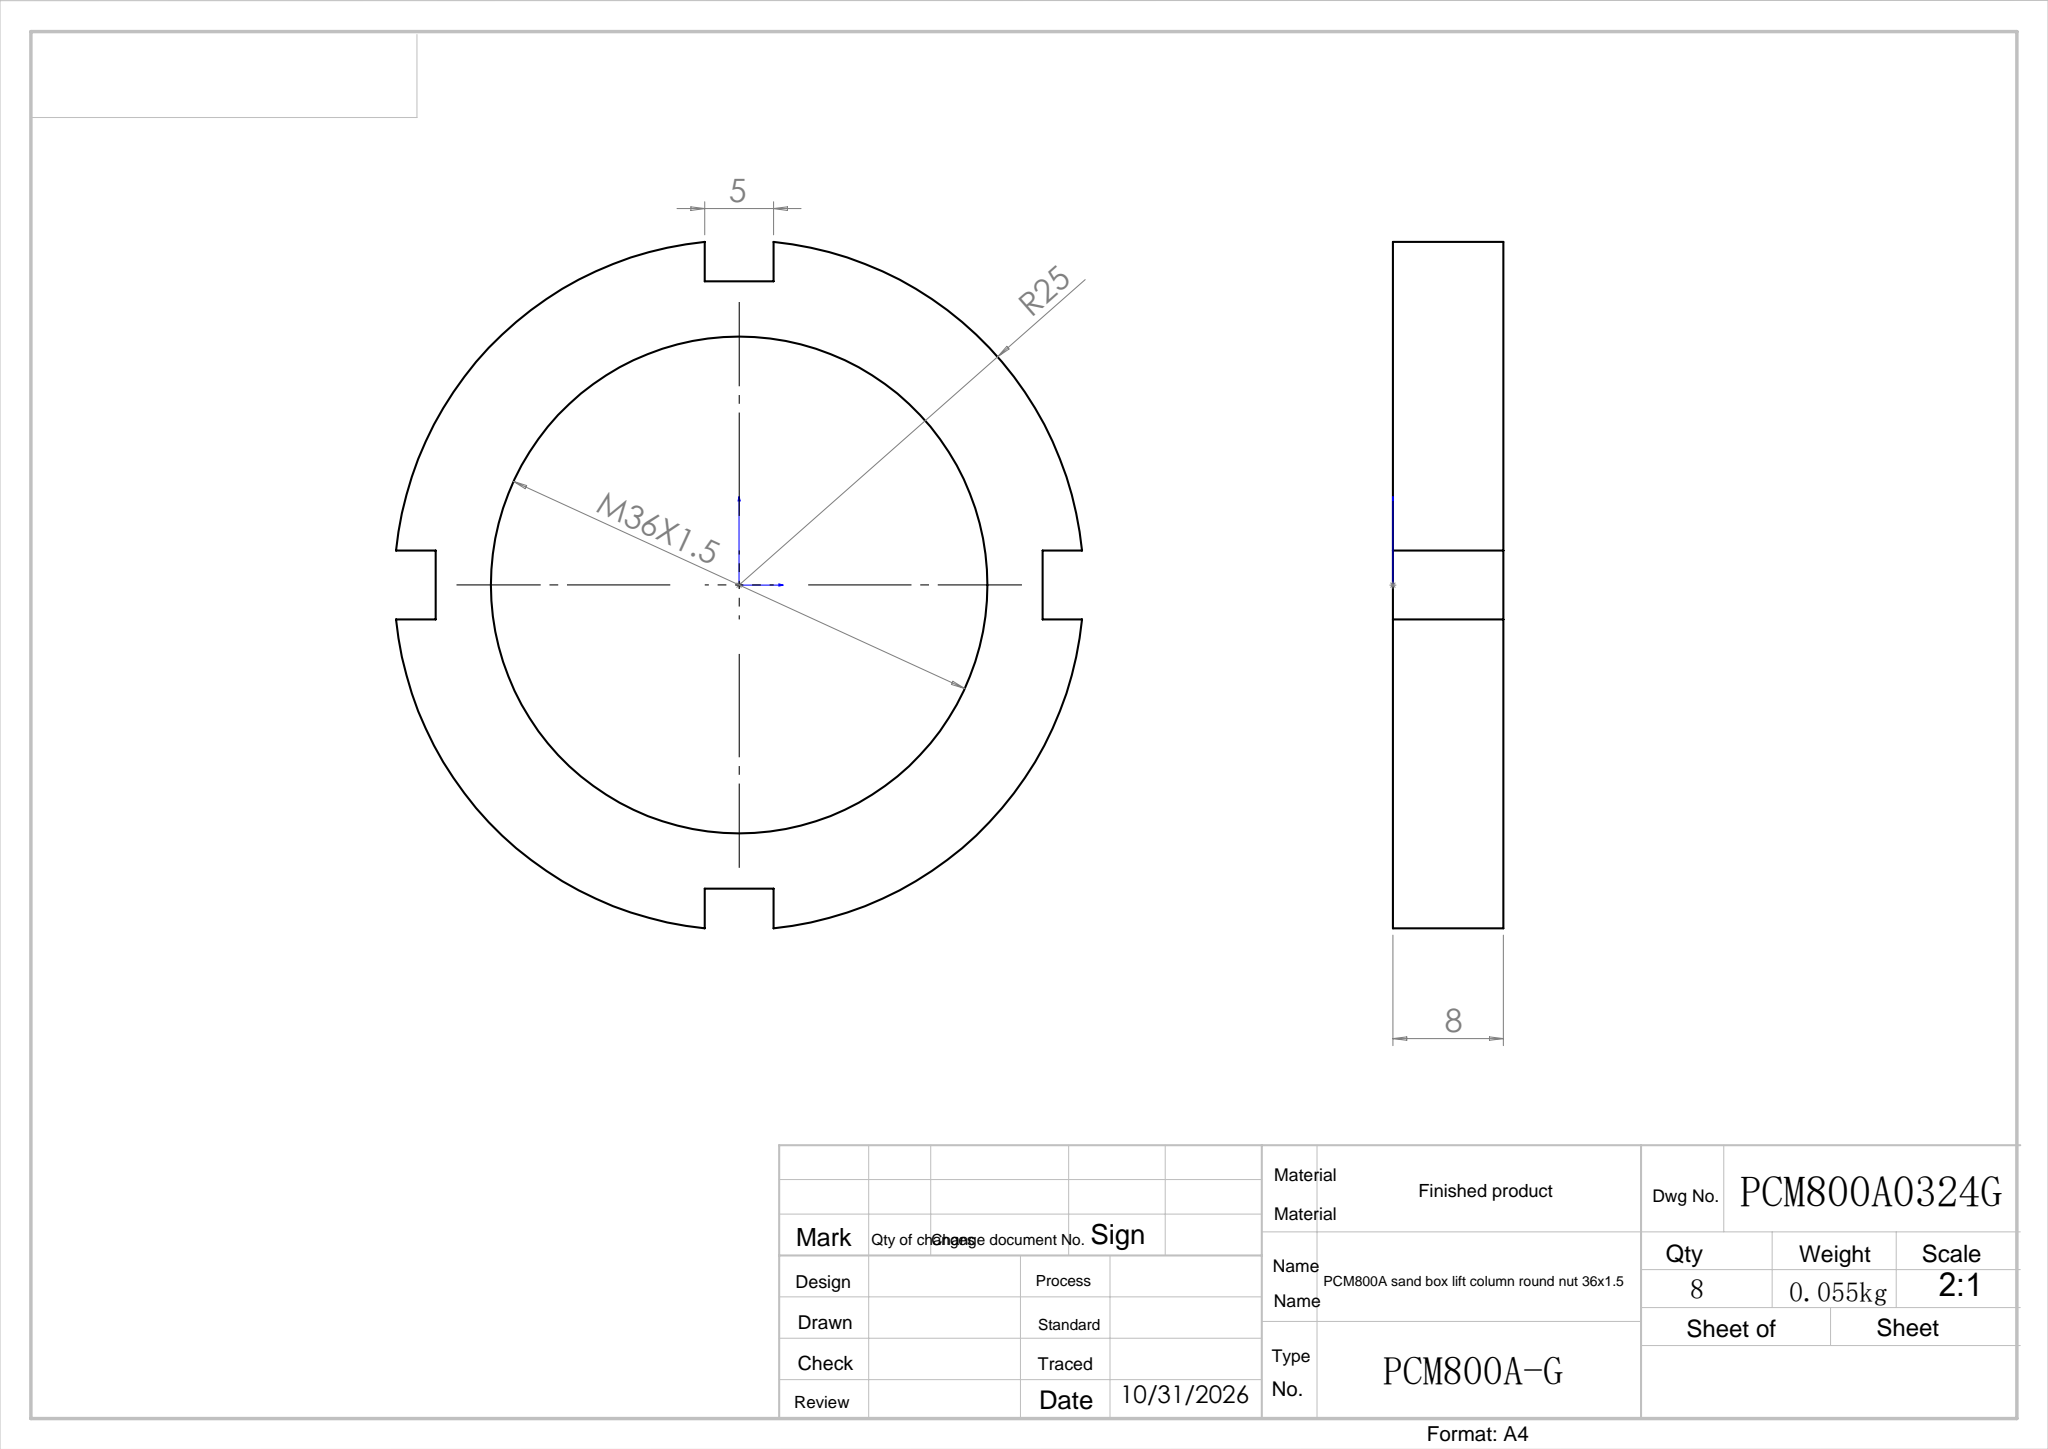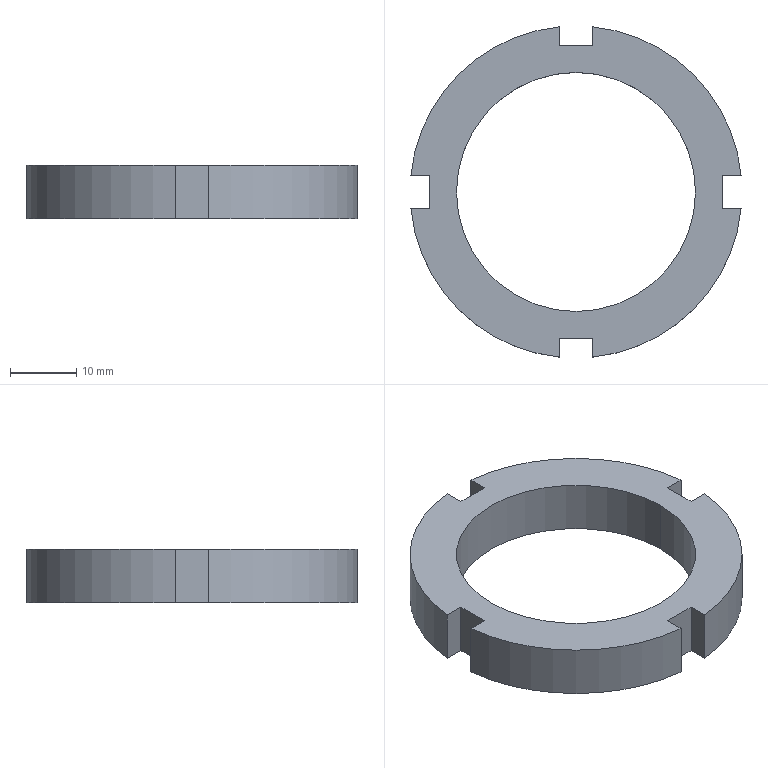Part | SolidWorks | features Extrusion 1 | 1 solid | 20 faces | box 49.742 x 49.742 x 8 mm | volume 7088 mm3 | plane 14 | cylinder 6 | commonest cylinder face diameters 49.993 x4 36 x2
STEP:
#1=CARTESIAN_POINT('',(-18.,0.,8.));
#2=VERTEX_POINT('',#1);
#3=CARTESIAN_POINT('',(18.,0.,8.));
#4=VERTEX_POINT('',#3);
#5=CARTESIAN_POINT('',(0.,0.,8.));
#6=DIRECTION('',(0.,0.,1.));
#7=DIRECTION('',(1.,0.,0.));
#8=AXIS2_PLACEMENT_3D('',#5,#6,#7);
#9=CIRCLE('',#8,18.);
#10=EDGE_CURVE('',#2,#4,#9,.T.);
#11=ORIENTED_EDGE('',*,*,#10,.T.);
#12=CARTESIAN_POINT('',(18.,0.,0.));
#13=VERTEX_POINT('',#12);
#14=CARTESIAN_POINT('',(18.,0.,8.));
#15=DIRECTION('',(0.,0.,-1.));
#16=VECTOR('',#15,1000.);
#17=LINE('',#14,#16);
#18=EDGE_CURVE('',#4,#13,#17,.T.);
#19=ORIENTED_EDGE('',*,*,#18,.T.);
#20=CARTESIAN_POINT('',(-18.,0.,0.));
#21=VERTEX_POINT('',#20);
#22=CARTESIAN_POINT('',(0.,0.,0.));
#23=DIRECTION('',(0.,0.,1.));
#24=DIRECTION('',(1.,0.,0.));
#25=AXIS2_PLACEMENT_3D('',#22,#23,#24);
#26=CIRCLE('',#25,18.);
#27=EDGE_CURVE('',#21,#13,#26,.T.);
#28=ORIENTED_EDGE('',*,*,#27,.F.);
#29=CARTESIAN_POINT('',(-18.,0.,8.));
#30=DIRECTION('',(0.,0.,-1.));
#31=VECTOR('',#30,1000.);
#32=LINE('',#29,#31);
#33=EDGE_CURVE('',#2,#21,#32,.T.);
#34=ORIENTED_EDGE('',*,*,#33,.F.);
#35=EDGE_LOOP('',(#11,#19,#28,#34));
#36=FACE_OUTER_BOUND('',#35,.T.);
#37=CARTESIAN_POINT('',(0.,0.,8.));
#38=DIRECTION('',(0.,0.,-1.));
#39=DIRECTION('',(-1.,0.,0.));
#40=AXIS2_PLACEMENT_3D('',#37,#38,#39);
#41=CYLINDRICAL_SURFACE('',#40,18.);
#42=ADVANCED_FACE('',(#36),#41,.F.);
#43=CARTESIAN_POINT('',(-2.5,24.871,8.));
#44=VERTEX_POINT('',#43);
#45=CARTESIAN_POINT('',(-24.871,2.5,8.));
#46=VERTEX_POINT('',#45);
#47=CARTESIAN_POINT('',(0.,0.,8.));
#48=DIRECTION('',(0.,0.,1.));
#49=DIRECTION('',(1.,0.,0.));
#50=AXIS2_PLACEMENT_3D('',#47,#48,#49);
#51=CIRCLE('',#50,24.996);
#52=EDGE_CURVE('',#44,#46,#51,.T.);
#53=ORIENTED_EDGE('',*,*,#52,.T.);
#54=CARTESIAN_POINT('',(-22.,2.5,8.));
#55=VERTEX_POINT('',#54);
#56=CARTESIAN_POINT('',(-22.,2.5,8.));
#57=DIRECTION('',(1.,0.,0.));
#58=VECTOR('',#57,1000.);
#59=LINE('',#56,#58);
#60=EDGE_CURVE('',#46,#55,#59,.T.);
#61=ORIENTED_EDGE('',*,*,#60,.T.);
#62=CARTESIAN_POINT('',(-22.,-2.5,8.));
#63=VERTEX_POINT('',#62);
#64=CARTESIAN_POINT('',(-22.,-2.5,8.));
#65=DIRECTION('',(0.,-1.,0.));
#66=VECTOR('',#65,1000.);
#67=LINE('',#64,#66);
#68=EDGE_CURVE('',#55,#63,#67,.T.);
#69=ORIENTED_EDGE('',*,*,#68,.T.);
#70=CARTESIAN_POINT('',(-24.871,-2.5,8.));
#71=VERTEX_POINT('',#70);
#72=CARTESIAN_POINT('',(-24.871,-2.5,8.));
#73=DIRECTION('',(-1.,0.,0.));
#74=VECTOR('',#73,1000.);
#75=LINE('',#72,#74);
#76=EDGE_CURVE('',#63,#71,#75,.T.);
#77=ORIENTED_EDGE('',*,*,#76,.T.);
#78=CARTESIAN_POINT('',(-2.5,-24.871,8.));
#79=VERTEX_POINT('',#78);
#80=CARTESIAN_POINT('',(0.,0.,8.));
#81=DIRECTION('',(0.,0.,1.));
#82=DIRECTION('',(1.,0.,0.));
#83=AXIS2_PLACEMENT_3D('',#80,#81,#82);
#84=CIRCLE('',#83,24.996);
#85=EDGE_CURVE('',#71,#79,#84,.T.);
#86=ORIENTED_EDGE('',*,*,#85,.T.);
#87=CARTESIAN_POINT('',(-2.5,-22.,8.));
#88=VERTEX_POINT('',#87);
#89=CARTESIAN_POINT('',(-2.5,-22.,8.));
#90=DIRECTION('',(0.,1.,0.));
#91=VECTOR('',#90,1000.);
#92=LINE('',#89,#91);
#93=EDGE_CURVE('',#79,#88,#92,.T.);
#94=ORIENTED_EDGE('',*,*,#93,.T.);
#95=CARTESIAN_POINT('',(2.5,-22.,8.));
#96=VERTEX_POINT('',#95);
#97=CARTESIAN_POINT('',(2.5,-22.,8.));
#98=DIRECTION('',(1.,0.,0.));
#99=VECTOR('',#98,1000.);
#100=LINE('',#97,#99);
#101=EDGE_CURVE('',#88,#96,#100,.T.);
#102=ORIENTED_EDGE('',*,*,#101,.T.);
#103=CARTESIAN_POINT('',(2.5,-24.871,8.));
#104=VERTEX_POINT('',#103);
#105=CARTESIAN_POINT('',(2.5,-24.871,8.));
#106=DIRECTION('',(0.,-1.,0.));
#107=VECTOR('',#106,1000.);
#108=LINE('',#105,#107);
#109=EDGE_CURVE('',#96,#104,#108,.T.);
#110=ORIENTED_EDGE('',*,*,#109,.T.);
#111=CARTESIAN_POINT('',(24.871,-2.5,8.));
#112=VERTEX_POINT('',#111);
#113=CARTESIAN_POINT('',(0.,0.,8.));
#114=DIRECTION('',(0.,0.,1.));
#115=DIRECTION('',(1.,0.,0.));
#116=AXIS2_PLACEMENT_3D('',#113,#114,#115);
#117=CIRCLE('',#116,24.996);
#118=EDGE_CURVE('',#104,#112,#117,.T.);
#119=ORIENTED_EDGE('',*,*,#118,.T.);
#120=CARTESIAN_POINT('',(22.,-2.5,8.));
#121=VERTEX_POINT('',#120);
#122=CARTESIAN_POINT('',(22.,-2.5,8.));
#123=DIRECTION('',(-1.,0.,0.));
#124=VECTOR('',#123,1000.);
#125=LINE('',#122,#124);
#126=EDGE_CURVE('',#112,#121,#125,.T.);
#127=ORIENTED_EDGE('',*,*,#126,.T.);
#128=CARTESIAN_POINT('',(22.,2.5,8.));
#129=VERTEX_POINT('',#128);
#130=CARTESIAN_POINT('',(22.,2.5,8.));
#131=DIRECTION('',(0.,1.,0.));
#132=VECTOR('',#131,1000.);
#133=LINE('',#130,#132);
#134=EDGE_CURVE('',#121,#129,#133,.T.);
#135=ORIENTED_EDGE('',*,*,#134,.T.);
#136=CARTESIAN_POINT('',(24.871,2.5,8.));
#137=VERTEX_POINT('',#136);
#138=CARTESIAN_POINT('',(24.871,2.5,8.));
#139=DIRECTION('',(1.,0.,0.));
#140=VECTOR('',#139,1000.);
#141=LINE('',#138,#140);
#142=EDGE_CURVE('',#129,#137,#141,.T.);
#143=ORIENTED_EDGE('',*,*,#142,.T.);
#144=CARTESIAN_POINT('',(2.5,24.871,8.));
#145=VERTEX_POINT('',#144);
#146=CARTESIAN_POINT('',(0.,0.,8.));
#147=DIRECTION('',(0.,0.,1.));
#148=DIRECTION('',(1.,0.,0.));
#149=AXIS2_PLACEMENT_3D('',#146,#147,#148);
#150=CIRCLE('',#149,24.996);
#151=EDGE_CURVE('',#137,#145,#150,.T.);
#152=ORIENTED_EDGE('',*,*,#151,.T.);
#153=CARTESIAN_POINT('',(2.5,22.,8.));
#154=VERTEX_POINT('',#153);
#155=CARTESIAN_POINT('',(2.5,22.,8.));
#156=DIRECTION('',(0.,-1.,0.));
#157=VECTOR('',#156,1000.);
#158=LINE('',#155,#157);
#159=EDGE_CURVE('',#145,#154,#158,.T.);
#160=ORIENTED_EDGE('',*,*,#159,.T.);
#161=CARTESIAN_POINT('',(-2.5,22.,8.));
#162=VERTEX_POINT('',#161);
#163=CARTESIAN_POINT('',(-2.5,22.,8.));
#164=DIRECTION('',(-1.,0.,0.));
#165=VECTOR('',#164,1000.);
#166=LINE('',#163,#165);
#167=EDGE_CURVE('',#154,#162,#166,.T.);
#168=ORIENTED_EDGE('',*,*,#167,.T.);
#169=CARTESIAN_POINT('',(-2.5,24.871,8.));
#170=DIRECTION('',(0.,1.,0.));
#171=VECTOR('',#170,1000.);
#172=LINE('',#169,#171);
#173=EDGE_CURVE('',#162,#44,#172,.T.);
#174=ORIENTED_EDGE('',*,*,#173,.T.);
#175=EDGE_LOOP('',(#53,#61,#69,#77,#86,#94,#102,#110,#119,#127,#135,#143,#152,#160,#168,#174));
#176=FACE_OUTER_BOUND('',#175,.T.);
#177=ORIENTED_EDGE('',*,*,#10,.F.);
#178=CARTESIAN_POINT('',(0.,0.,8.));
#179=DIRECTION('',(0.,0.,1.));
#180=DIRECTION('',(1.,0.,0.));
#181=AXIS2_PLACEMENT_3D('',#178,#179,#180);
#182=CIRCLE('',#181,18.);
#183=EDGE_CURVE('',#4,#2,#182,.T.);
#184=ORIENTED_EDGE('',*,*,#183,.F.);
#185=EDGE_LOOP('',(#177,#184));
#186=FACE_BOUND('',#185,.T.);
#187=CARTESIAN_POINT('',(0.,0.,8.));
#188=DIRECTION('',(0.,0.,1.));
#189=DIRECTION('',(1.,0.,0.));
#190=AXIS2_PLACEMENT_3D('',#187,#188,#189);
#191=PLANE('',#190);
#192=ADVANCED_FACE('',(#176,#186),#191,.T.);
#193=CARTESIAN_POINT('',(-2.5,24.871,0.));
#194=VERTEX_POINT('',#193);
#195=CARTESIAN_POINT('',(-24.871,2.5,0.));
#196=VERTEX_POINT('',#195);
#197=CARTESIAN_POINT('',(0.,0.,0.));
#198=DIRECTION('',(0.,0.,1.));
#199=DIRECTION('',(1.,0.,0.));
#200=AXIS2_PLACEMENT_3D('',#197,#198,#199);
#201=CIRCLE('',#200,24.996);
#202=EDGE_CURVE('',#194,#196,#201,.T.);
#203=ORIENTED_EDGE('',*,*,#202,.F.);
#204=CARTESIAN_POINT('',(-2.5,22.,0.));
#205=VERTEX_POINT('',#204);
#206=CARTESIAN_POINT('',(-2.5,24.871,0.));
#207=DIRECTION('',(0.,1.,0.));
#208=VECTOR('',#207,1000.);
#209=LINE('',#206,#208);
#210=EDGE_CURVE('',#205,#194,#209,.T.);
#211=ORIENTED_EDGE('',*,*,#210,.F.);
#212=CARTESIAN_POINT('',(2.5,22.,0.));
#213=VERTEX_POINT('',#212);
#214=CARTESIAN_POINT('',(-2.5,22.,0.));
#215=DIRECTION('',(-1.,0.,0.));
#216=VECTOR('',#215,1000.);
#217=LINE('',#214,#216);
#218=EDGE_CURVE('',#213,#205,#217,.T.);
#219=ORIENTED_EDGE('',*,*,#218,.F.);
#220=CARTESIAN_POINT('',(2.5,24.871,0.));
#221=VERTEX_POINT('',#220);
#222=CARTESIAN_POINT('',(2.5,22.,0.));
#223=DIRECTION('',(0.,-1.,0.));
#224=VECTOR('',#223,1000.);
#225=LINE('',#222,#224);
#226=EDGE_CURVE('',#221,#213,#225,.T.);
#227=ORIENTED_EDGE('',*,*,#226,.F.);
#228=CARTESIAN_POINT('',(24.871,2.5,0.));
#229=VERTEX_POINT('',#228);
#230=CARTESIAN_POINT('',(0.,0.,0.));
#231=DIRECTION('',(0.,0.,1.));
#232=DIRECTION('',(1.,0.,0.));
#233=AXIS2_PLACEMENT_3D('',#230,#231,#232);
#234=CIRCLE('',#233,24.996);
#235=EDGE_CURVE('',#229,#221,#234,.T.);
#236=ORIENTED_EDGE('',*,*,#235,.F.);
#237=CARTESIAN_POINT('',(22.,2.5,0.));
#238=VERTEX_POINT('',#237);
#239=CARTESIAN_POINT('',(24.871,2.5,0.));
#240=DIRECTION('',(1.,0.,0.));
#241=VECTOR('',#240,1000.);
#242=LINE('',#239,#241);
#243=EDGE_CURVE('',#238,#229,#242,.T.);
#244=ORIENTED_EDGE('',*,*,#243,.F.);
#245=CARTESIAN_POINT('',(22.,-2.5,0.));
#246=VERTEX_POINT('',#245);
#247=CARTESIAN_POINT('',(22.,2.5,0.));
#248=DIRECTION('',(0.,1.,0.));
#249=VECTOR('',#248,1000.);
#250=LINE('',#247,#249);
#251=EDGE_CURVE('',#246,#238,#250,.T.);
#252=ORIENTED_EDGE('',*,*,#251,.F.);
#253=CARTESIAN_POINT('',(24.871,-2.5,0.));
#254=VERTEX_POINT('',#253);
#255=CARTESIAN_POINT('',(22.,-2.5,0.));
#256=DIRECTION('',(-1.,0.,0.));
#257=VECTOR('',#256,1000.);
#258=LINE('',#255,#257);
#259=EDGE_CURVE('',#254,#246,#258,.T.);
#260=ORIENTED_EDGE('',*,*,#259,.F.);
#261=CARTESIAN_POINT('',(2.5,-24.871,0.));
#262=VERTEX_POINT('',#261);
#263=CARTESIAN_POINT('',(0.,0.,0.));
#264=DIRECTION('',(0.,0.,1.));
#265=DIRECTION('',(1.,0.,0.));
#266=AXIS2_PLACEMENT_3D('',#263,#264,#265);
#267=CIRCLE('',#266,24.996);
#268=EDGE_CURVE('',#262,#254,#267,.T.);
#269=ORIENTED_EDGE('',*,*,#268,.F.);
#270=CARTESIAN_POINT('',(2.5,-22.,0.));
#271=VERTEX_POINT('',#270);
#272=CARTESIAN_POINT('',(2.5,-24.871,0.));
#273=DIRECTION('',(0.,-1.,0.));
#274=VECTOR('',#273,1000.);
#275=LINE('',#272,#274);
#276=EDGE_CURVE('',#271,#262,#275,.T.);
#277=ORIENTED_EDGE('',*,*,#276,.F.);
#278=CARTESIAN_POINT('',(-2.5,-22.,0.));
#279=VERTEX_POINT('',#278);
#280=CARTESIAN_POINT('',(2.5,-22.,0.));
#281=DIRECTION('',(1.,0.,0.));
#282=VECTOR('',#281,1000.);
#283=LINE('',#280,#282);
#284=EDGE_CURVE('',#279,#271,#283,.T.);
#285=ORIENTED_EDGE('',*,*,#284,.F.);
#286=CARTESIAN_POINT('',(-2.5,-24.871,0.));
#287=VERTEX_POINT('',#286);
#288=CARTESIAN_POINT('',(-2.5,-22.,0.));
#289=DIRECTION('',(0.,1.,0.));
#290=VECTOR('',#289,1000.);
#291=LINE('',#288,#290);
#292=EDGE_CURVE('',#287,#279,#291,.T.);
#293=ORIENTED_EDGE('',*,*,#292,.F.);
#294=CARTESIAN_POINT('',(-24.871,-2.5,0.));
#295=VERTEX_POINT('',#294);
#296=CARTESIAN_POINT('',(0.,0.,0.));
#297=DIRECTION('',(0.,0.,1.));
#298=DIRECTION('',(1.,0.,0.));
#299=AXIS2_PLACEMENT_3D('',#296,#297,#298);
#300=CIRCLE('',#299,24.996);
#301=EDGE_CURVE('',#295,#287,#300,.T.);
#302=ORIENTED_EDGE('',*,*,#301,.F.);
#303=CARTESIAN_POINT('',(-22.,-2.5,0.));
#304=VERTEX_POINT('',#303);
#305=CARTESIAN_POINT('',(-24.871,-2.5,0.));
#306=DIRECTION('',(-1.,0.,0.));
#307=VECTOR('',#306,1000.);
#308=LINE('',#305,#307);
#309=EDGE_CURVE('',#304,#295,#308,.T.);
#310=ORIENTED_EDGE('',*,*,#309,.F.);
#311=CARTESIAN_POINT('',(-22.,2.5,0.));
#312=VERTEX_POINT('',#311);
#313=CARTESIAN_POINT('',(-22.,-2.5,0.));
#314=DIRECTION('',(0.,-1.,0.));
#315=VECTOR('',#314,1000.);
#316=LINE('',#313,#315);
#317=EDGE_CURVE('',#312,#304,#316,.T.);
#318=ORIENTED_EDGE('',*,*,#317,.F.);
#319=CARTESIAN_POINT('',(-22.,2.5,0.));
#320=DIRECTION('',(1.,0.,0.));
#321=VECTOR('',#320,1000.);
#322=LINE('',#319,#321);
#323=EDGE_CURVE('',#196,#312,#322,.T.);
#324=ORIENTED_EDGE('',*,*,#323,.F.);
#325=EDGE_LOOP('',(#203,#211,#219,#227,#236,#244,#252,#260,#269,#277,#285,#293,#302,#310,#318,#324));
#326=FACE_OUTER_BOUND('',#325,.T.);
#327=ORIENTED_EDGE('',*,*,#27,.T.);
#328=CARTESIAN_POINT('',(0.,0.,0.));
#329=DIRECTION('',(0.,0.,1.));
#330=DIRECTION('',(1.,0.,0.));
#331=AXIS2_PLACEMENT_3D('',#328,#329,#330);
#332=CIRCLE('',#331,18.);
#333=EDGE_CURVE('',#13,#21,#332,.T.);
#334=ORIENTED_EDGE('',*,*,#333,.T.);
#335=EDGE_LOOP('',(#327,#334));
#336=FACE_BOUND('',#335,.T.);
#337=CARTESIAN_POINT('',(0.,0.,0.));
#338=DIRECTION('',(0.,0.,1.));
#339=DIRECTION('',(1.,0.,0.));
#340=AXIS2_PLACEMENT_3D('',#337,#338,#339);
#341=PLANE('',#340);
#342=ADVANCED_FACE('',(#326,#336),#341,.F.);
#343=ORIENTED_EDGE('',*,*,#202,.T.);
#344=CARTESIAN_POINT('',(-24.871,2.5,8.));
#345=DIRECTION('',(0.,0.,-1.));
#346=VECTOR('',#345,1000.);
#347=LINE('',#344,#346);
#348=EDGE_CURVE('',#46,#196,#347,.T.);
#349=ORIENTED_EDGE('',*,*,#348,.F.);
#350=ORIENTED_EDGE('',*,*,#52,.F.);
#351=CARTESIAN_POINT('',(-2.5,24.871,8.));
#352=DIRECTION('',(0.,0.,-1.));
#353=VECTOR('',#352,1000.);
#354=LINE('',#351,#353);
#355=EDGE_CURVE('',#44,#194,#354,.T.);
#356=ORIENTED_EDGE('',*,*,#355,.T.);
#357=EDGE_LOOP('',(#343,#349,#350,#356));
#358=FACE_OUTER_BOUND('',#357,.T.);
#359=CARTESIAN_POINT('',(0.,0.,8.));
#360=DIRECTION('',(0.,0.,-1.));
#361=DIRECTION('',(-1.,0.,0.));
#362=AXIS2_PLACEMENT_3D('',#359,#360,#361);
#363=CYLINDRICAL_SURFACE('',#362,24.996);
#364=ADVANCED_FACE('',(#358),#363,.T.);
#365=ORIENTED_EDGE('',*,*,#323,.T.);
#366=CARTESIAN_POINT('',(-22.,2.5,8.));
#367=DIRECTION('',(0.,0.,-1.));
#368=VECTOR('',#367,1000.);
#369=LINE('',#366,#368);
#370=EDGE_CURVE('',#55,#312,#369,.T.);
#371=ORIENTED_EDGE('',*,*,#370,.F.);
#372=ORIENTED_EDGE('',*,*,#60,.F.);
#373=ORIENTED_EDGE('',*,*,#348,.T.);
#374=EDGE_LOOP('',(#365,#371,#372,#373));
#375=FACE_OUTER_BOUND('',#374,.T.);
#376=CARTESIAN_POINT('',(-22.,2.5,8.));
#377=DIRECTION('',(0.,1.,0.));
#378=DIRECTION('',(-1.,0.,0.));
#379=AXIS2_PLACEMENT_3D('',#376,#377,#378);
#380=PLANE('',#379);
#381=ADVANCED_FACE('',(#375),#380,.F.);
#382=ORIENTED_EDGE('',*,*,#317,.T.);
#383=CARTESIAN_POINT('',(-22.,-2.5,8.));
#384=DIRECTION('',(0.,0.,-1.));
#385=VECTOR('',#384,1000.);
#386=LINE('',#383,#385);
#387=EDGE_CURVE('',#63,#304,#386,.T.);
#388=ORIENTED_EDGE('',*,*,#387,.F.);
#389=ORIENTED_EDGE('',*,*,#68,.F.);
#390=ORIENTED_EDGE('',*,*,#370,.T.);
#391=EDGE_LOOP('',(#382,#388,#389,#390));
#392=FACE_OUTER_BOUND('',#391,.T.);
#393=CARTESIAN_POINT('',(-22.,-2.5,8.));
#394=DIRECTION('',(1.,0.,0.));
#395=DIRECTION('',(0.,1.,0.));
#396=AXIS2_PLACEMENT_3D('',#393,#394,#395);
#397=PLANE('',#396);
#398=ADVANCED_FACE('',(#392),#397,.F.);
#399=ORIENTED_EDGE('',*,*,#309,.T.);
#400=CARTESIAN_POINT('',(-24.871,-2.5,8.));
#401=DIRECTION('',(0.,0.,-1.));
#402=VECTOR('',#401,1000.);
#403=LINE('',#400,#402);
#404=EDGE_CURVE('',#71,#295,#403,.T.);
#405=ORIENTED_EDGE('',*,*,#404,.F.);
#406=ORIENTED_EDGE('',*,*,#76,.F.);
#407=ORIENTED_EDGE('',*,*,#387,.T.);
#408=EDGE_LOOP('',(#399,#405,#406,#407));
#409=FACE_OUTER_BOUND('',#408,.T.);
#410=CARTESIAN_POINT('',(-24.871,-2.5,8.));
#411=DIRECTION('',(0.,-1.,0.));
#412=DIRECTION('',(1.,0.,0.));
#413=AXIS2_PLACEMENT_3D('',#410,#411,#412);
#414=PLANE('',#413);
#415=ADVANCED_FACE('',(#409),#414,.F.);
#416=ORIENTED_EDGE('',*,*,#301,.T.);
#417=CARTESIAN_POINT('',(-2.5,-24.871,8.));
#418=DIRECTION('',(0.,0.,-1.));
#419=VECTOR('',#418,1000.);
#420=LINE('',#417,#419);
#421=EDGE_CURVE('',#79,#287,#420,.T.);
#422=ORIENTED_EDGE('',*,*,#421,.F.);
#423=ORIENTED_EDGE('',*,*,#85,.F.);
#424=ORIENTED_EDGE('',*,*,#404,.T.);
#425=EDGE_LOOP('',(#416,#422,#423,#424));
#426=FACE_OUTER_BOUND('',#425,.T.);
#427=CARTESIAN_POINT('',(0.,0.,8.));
#428=DIRECTION('',(0.,0.,-1.));
#429=DIRECTION('',(-1.,0.,0.));
#430=AXIS2_PLACEMENT_3D('',#427,#428,#429);
#431=CYLINDRICAL_SURFACE('',#430,24.996);
#432=ADVANCED_FACE('',(#426),#431,.T.);
#433=ORIENTED_EDGE('',*,*,#292,.T.);
#434=CARTESIAN_POINT('',(-2.5,-22.,8.));
#435=DIRECTION('',(0.,0.,-1.));
#436=VECTOR('',#435,1000.);
#437=LINE('',#434,#436);
#438=EDGE_CURVE('',#88,#279,#437,.T.);
#439=ORIENTED_EDGE('',*,*,#438,.F.);
#440=ORIENTED_EDGE('',*,*,#93,.F.);
#441=ORIENTED_EDGE('',*,*,#421,.T.);
#442=EDGE_LOOP('',(#433,#439,#440,#441));
#443=FACE_OUTER_BOUND('',#442,.T.);
#444=CARTESIAN_POINT('',(-2.5,-22.,8.));
#445=DIRECTION('',(-1.,0.,0.));
#446=DIRECTION('',(0.,-1.,0.));
#447=AXIS2_PLACEMENT_3D('',#444,#445,#446);
#448=PLANE('',#447);
#449=ADVANCED_FACE('',(#443),#448,.F.);
#450=ORIENTED_EDGE('',*,*,#284,.T.);
#451=CARTESIAN_POINT('',(2.5,-22.,8.));
#452=DIRECTION('',(0.,0.,-1.));
#453=VECTOR('',#452,1000.);
#454=LINE('',#451,#453);
#455=EDGE_CURVE('',#96,#271,#454,.T.);
#456=ORIENTED_EDGE('',*,*,#455,.F.);
#457=ORIENTED_EDGE('',*,*,#101,.F.);
#458=ORIENTED_EDGE('',*,*,#438,.T.);
#459=EDGE_LOOP('',(#450,#456,#457,#458));
#460=FACE_OUTER_BOUND('',#459,.T.);
#461=CARTESIAN_POINT('',(2.5,-22.,8.));
#462=DIRECTION('',(0.,1.,0.));
#463=DIRECTION('',(-1.,0.,0.));
#464=AXIS2_PLACEMENT_3D('',#461,#462,#463);
#465=PLANE('',#464);
#466=ADVANCED_FACE('',(#460),#465,.F.);
#467=ORIENTED_EDGE('',*,*,#276,.T.);
#468=CARTESIAN_POINT('',(2.5,-24.871,8.));
#469=DIRECTION('',(0.,0.,-1.));
#470=VECTOR('',#469,1000.);
#471=LINE('',#468,#470);
#472=EDGE_CURVE('',#104,#262,#471,.T.);
#473=ORIENTED_EDGE('',*,*,#472,.F.);
#474=ORIENTED_EDGE('',*,*,#109,.F.);
#475=ORIENTED_EDGE('',*,*,#455,.T.);
#476=EDGE_LOOP('',(#467,#473,#474,#475));
#477=FACE_OUTER_BOUND('',#476,.T.);
#478=CARTESIAN_POINT('',(2.5,-24.871,8.));
#479=DIRECTION('',(1.,0.,0.));
#480=DIRECTION('',(0.,1.,0.));
#481=AXIS2_PLACEMENT_3D('',#478,#479,#480);
#482=PLANE('',#481);
#483=ADVANCED_FACE('',(#477),#482,.F.);
#484=ORIENTED_EDGE('',*,*,#268,.T.);
#485=CARTESIAN_POINT('',(24.871,-2.5,8.));
#486=DIRECTION('',(0.,0.,-1.));
#487=VECTOR('',#486,1000.);
#488=LINE('',#485,#487);
#489=EDGE_CURVE('',#112,#254,#488,.T.);
#490=ORIENTED_EDGE('',*,*,#489,.F.);
#491=ORIENTED_EDGE('',*,*,#118,.F.);
#492=ORIENTED_EDGE('',*,*,#472,.T.);
#493=EDGE_LOOP('',(#484,#490,#491,#492));
#494=FACE_OUTER_BOUND('',#493,.T.);
#495=CARTESIAN_POINT('',(0.,0.,8.));
#496=DIRECTION('',(0.,0.,-1.));
#497=DIRECTION('',(-1.,0.,0.));
#498=AXIS2_PLACEMENT_3D('',#495,#496,#497);
#499=CYLINDRICAL_SURFACE('',#498,24.996);
#500=ADVANCED_FACE('',(#494),#499,.T.);
#501=ORIENTED_EDGE('',*,*,#259,.T.);
#502=CARTESIAN_POINT('',(22.,-2.5,8.));
#503=DIRECTION('',(0.,0.,-1.));
#504=VECTOR('',#503,1000.);
#505=LINE('',#502,#504);
#506=EDGE_CURVE('',#121,#246,#505,.T.);
#507=ORIENTED_EDGE('',*,*,#506,.F.);
#508=ORIENTED_EDGE('',*,*,#126,.F.);
#509=ORIENTED_EDGE('',*,*,#489,.T.);
#510=EDGE_LOOP('',(#501,#507,#508,#509));
#511=FACE_OUTER_BOUND('',#510,.T.);
#512=CARTESIAN_POINT('',(22.,-2.5,8.));
#513=DIRECTION('',(0.,-1.,0.));
#514=DIRECTION('',(1.,0.,0.));
#515=AXIS2_PLACEMENT_3D('',#512,#513,#514);
#516=PLANE('',#515);
#517=ADVANCED_FACE('',(#511),#516,.F.);
#518=ORIENTED_EDGE('',*,*,#251,.T.);
#519=CARTESIAN_POINT('',(22.,2.5,8.));
#520=DIRECTION('',(0.,0.,-1.));
#521=VECTOR('',#520,1000.);
#522=LINE('',#519,#521);
#523=EDGE_CURVE('',#129,#238,#522,.T.);
#524=ORIENTED_EDGE('',*,*,#523,.F.);
#525=ORIENTED_EDGE('',*,*,#134,.F.);
#526=ORIENTED_EDGE('',*,*,#506,.T.);
#527=EDGE_LOOP('',(#518,#524,#525,#526));
#528=FACE_OUTER_BOUND('',#527,.T.);
#529=CARTESIAN_POINT('',(22.,2.5,8.));
#530=DIRECTION('',(-1.,0.,0.));
#531=DIRECTION('',(0.,-1.,0.));
#532=AXIS2_PLACEMENT_3D('',#529,#530,#531);
#533=PLANE('',#532);
#534=ADVANCED_FACE('',(#528),#533,.F.);
#535=ORIENTED_EDGE('',*,*,#243,.T.);
#536=CARTESIAN_POINT('',(24.871,2.5,8.));
#537=DIRECTION('',(0.,0.,-1.));
#538=VECTOR('',#537,1000.);
#539=LINE('',#536,#538);
#540=EDGE_CURVE('',#137,#229,#539,.T.);
#541=ORIENTED_EDGE('',*,*,#540,.F.);
#542=ORIENTED_EDGE('',*,*,#142,.F.);
#543=ORIENTED_EDGE('',*,*,#523,.T.);
#544=EDGE_LOOP('',(#535,#541,#542,#543));
#545=FACE_OUTER_BOUND('',#544,.T.);
#546=CARTESIAN_POINT('',(24.871,2.5,8.));
#547=DIRECTION('',(0.,1.,0.));
#548=DIRECTION('',(-1.,0.,0.));
#549=AXIS2_PLACEMENT_3D('',#546,#547,#548);
#550=PLANE('',#549);
#551=ADVANCED_FACE('',(#545),#550,.F.);
#552=ORIENTED_EDGE('',*,*,#235,.T.);
#553=CARTESIAN_POINT('',(2.5,24.871,8.));
#554=DIRECTION('',(0.,0.,-1.));
#555=VECTOR('',#554,1000.);
#556=LINE('',#553,#555);
#557=EDGE_CURVE('',#145,#221,#556,.T.);
#558=ORIENTED_EDGE('',*,*,#557,.F.);
#559=ORIENTED_EDGE('',*,*,#151,.F.);
#560=ORIENTED_EDGE('',*,*,#540,.T.);
#561=EDGE_LOOP('',(#552,#558,#559,#560));
#562=FACE_OUTER_BOUND('',#561,.T.);
#563=CARTESIAN_POINT('',(0.,0.,8.));
#564=DIRECTION('',(0.,0.,-1.));
#565=DIRECTION('',(-1.,0.,0.));
#566=AXIS2_PLACEMENT_3D('',#563,#564,#565);
#567=CYLINDRICAL_SURFACE('',#566,24.996);
#568=ADVANCED_FACE('',(#562),#567,.T.);
#569=ORIENTED_EDGE('',*,*,#226,.T.);
#570=CARTESIAN_POINT('',(2.5,22.,8.));
#571=DIRECTION('',(0.,0.,-1.));
#572=VECTOR('',#571,1000.);
#573=LINE('',#570,#572);
#574=EDGE_CURVE('',#154,#213,#573,.T.);
#575=ORIENTED_EDGE('',*,*,#574,.F.);
#576=ORIENTED_EDGE('',*,*,#159,.F.);
#577=ORIENTED_EDGE('',*,*,#557,.T.);
#578=EDGE_LOOP('',(#569,#575,#576,#577));
#579=FACE_OUTER_BOUND('',#578,.T.);
#580=CARTESIAN_POINT('',(2.5,22.,8.));
#581=DIRECTION('',(1.,0.,0.));
#582=DIRECTION('',(0.,1.,0.));
#583=AXIS2_PLACEMENT_3D('',#580,#581,#582);
#584=PLANE('',#583);
#585=ADVANCED_FACE('',(#579),#584,.F.);
#586=ORIENTED_EDGE('',*,*,#218,.T.);
#587=CARTESIAN_POINT('',(-2.5,22.,8.));
#588=DIRECTION('',(0.,0.,-1.));
#589=VECTOR('',#588,1000.);
#590=LINE('',#587,#589);
#591=EDGE_CURVE('',#162,#205,#590,.T.);
#592=ORIENTED_EDGE('',*,*,#591,.F.);
#593=ORIENTED_EDGE('',*,*,#167,.F.);
#594=ORIENTED_EDGE('',*,*,#574,.T.);
#595=EDGE_LOOP('',(#586,#592,#593,#594));
#596=FACE_OUTER_BOUND('',#595,.T.);
#597=CARTESIAN_POINT('',(-2.5,22.,8.));
#598=DIRECTION('',(0.,-1.,0.));
#599=DIRECTION('',(0.,0.,-1.));
#600=AXIS2_PLACEMENT_3D('',#597,#598,#599);
#601=PLANE('',#600);
#602=ADVANCED_FACE('',(#596),#601,.F.);
#603=ORIENTED_EDGE('',*,*,#210,.T.);
#604=ORIENTED_EDGE('',*,*,#355,.F.);
#605=ORIENTED_EDGE('',*,*,#173,.F.);
#606=ORIENTED_EDGE('',*,*,#591,.T.);
#607=EDGE_LOOP('',(#603,#604,#605,#606));
#608=FACE_OUTER_BOUND('',#607,.T.);
#609=CARTESIAN_POINT('',(-2.5,24.871,8.));
#610=DIRECTION('',(-1.,0.,0.));
#611=DIRECTION('',(0.,-1.,0.));
#612=AXIS2_PLACEMENT_3D('',#609,#610,#611);
#613=PLANE('',#612);
#614=ADVANCED_FACE('',(#608),#613,.F.);
#615=ORIENTED_EDGE('',*,*,#18,.F.);
#616=ORIENTED_EDGE('',*,*,#183,.T.);
#617=ORIENTED_EDGE('',*,*,#33,.T.);
#618=ORIENTED_EDGE('',*,*,#333,.F.);
#619=EDGE_LOOP('',(#615,#616,#617,#618));
#620=FACE_OUTER_BOUND('',#619,.T.);
#621=CARTESIAN_POINT('',(0.,0.,8.));
#622=DIRECTION('',(0.,0.,-1.));
#623=DIRECTION('',(-1.,0.,0.));
#624=AXIS2_PLACEMENT_3D('',#621,#622,#623);
#625=CYLINDRICAL_SURFACE('',#624,18.);
#626=ADVANCED_FACE('',(#620),#625,.F.);
#627=CLOSED_SHELL('',(#42,#192,#342,#364,#381,#398,#415,#432,#449,#466,#483,#500,#517,#534,#551,#568,#585,#602,#614,#626));
#628=MANIFOLD_SOLID_BREP('',#627);
#629=CARTESIAN_POINT('',(0.,0.,0.));
#630=DIRECTION('',(0.,0.,1.));
#631=DIRECTION('',(1.,0.,0.));
#632=AXIS2_PLACEMENT_3D('',#629,#630,#631);
#633=(LENGTH_UNIT()NAMED_UNIT(*)SI_UNIT(.MILLI.,.METRE.));
#634=UNCERTAINTY_MEASURE_WITH_UNIT(LENGTH_MEASURE(0.00001),#633,'','');
#635=(NAMED_UNIT(*)PLANE_ANGLE_UNIT()SI_UNIT($,.RADIAN.));
#636=(NAMED_UNIT(*)SI_UNIT($,.STERADIAN.)SOLID_ANGLE_UNIT());
#637=(GEOMETRIC_REPRESENTATION_CONTEXT(3)GLOBAL_UNCERTAINTY_ASSIGNED_CONTEXT((#634))GLOBAL_UNIT_ASSIGNED_CONTEXT((#633,#635,#636))REPRESENTATION_CONTEXT('',''));
#638=ADVANCED_BREP_SHAPE_REPRESENTATION('',(#628,#632),#637);